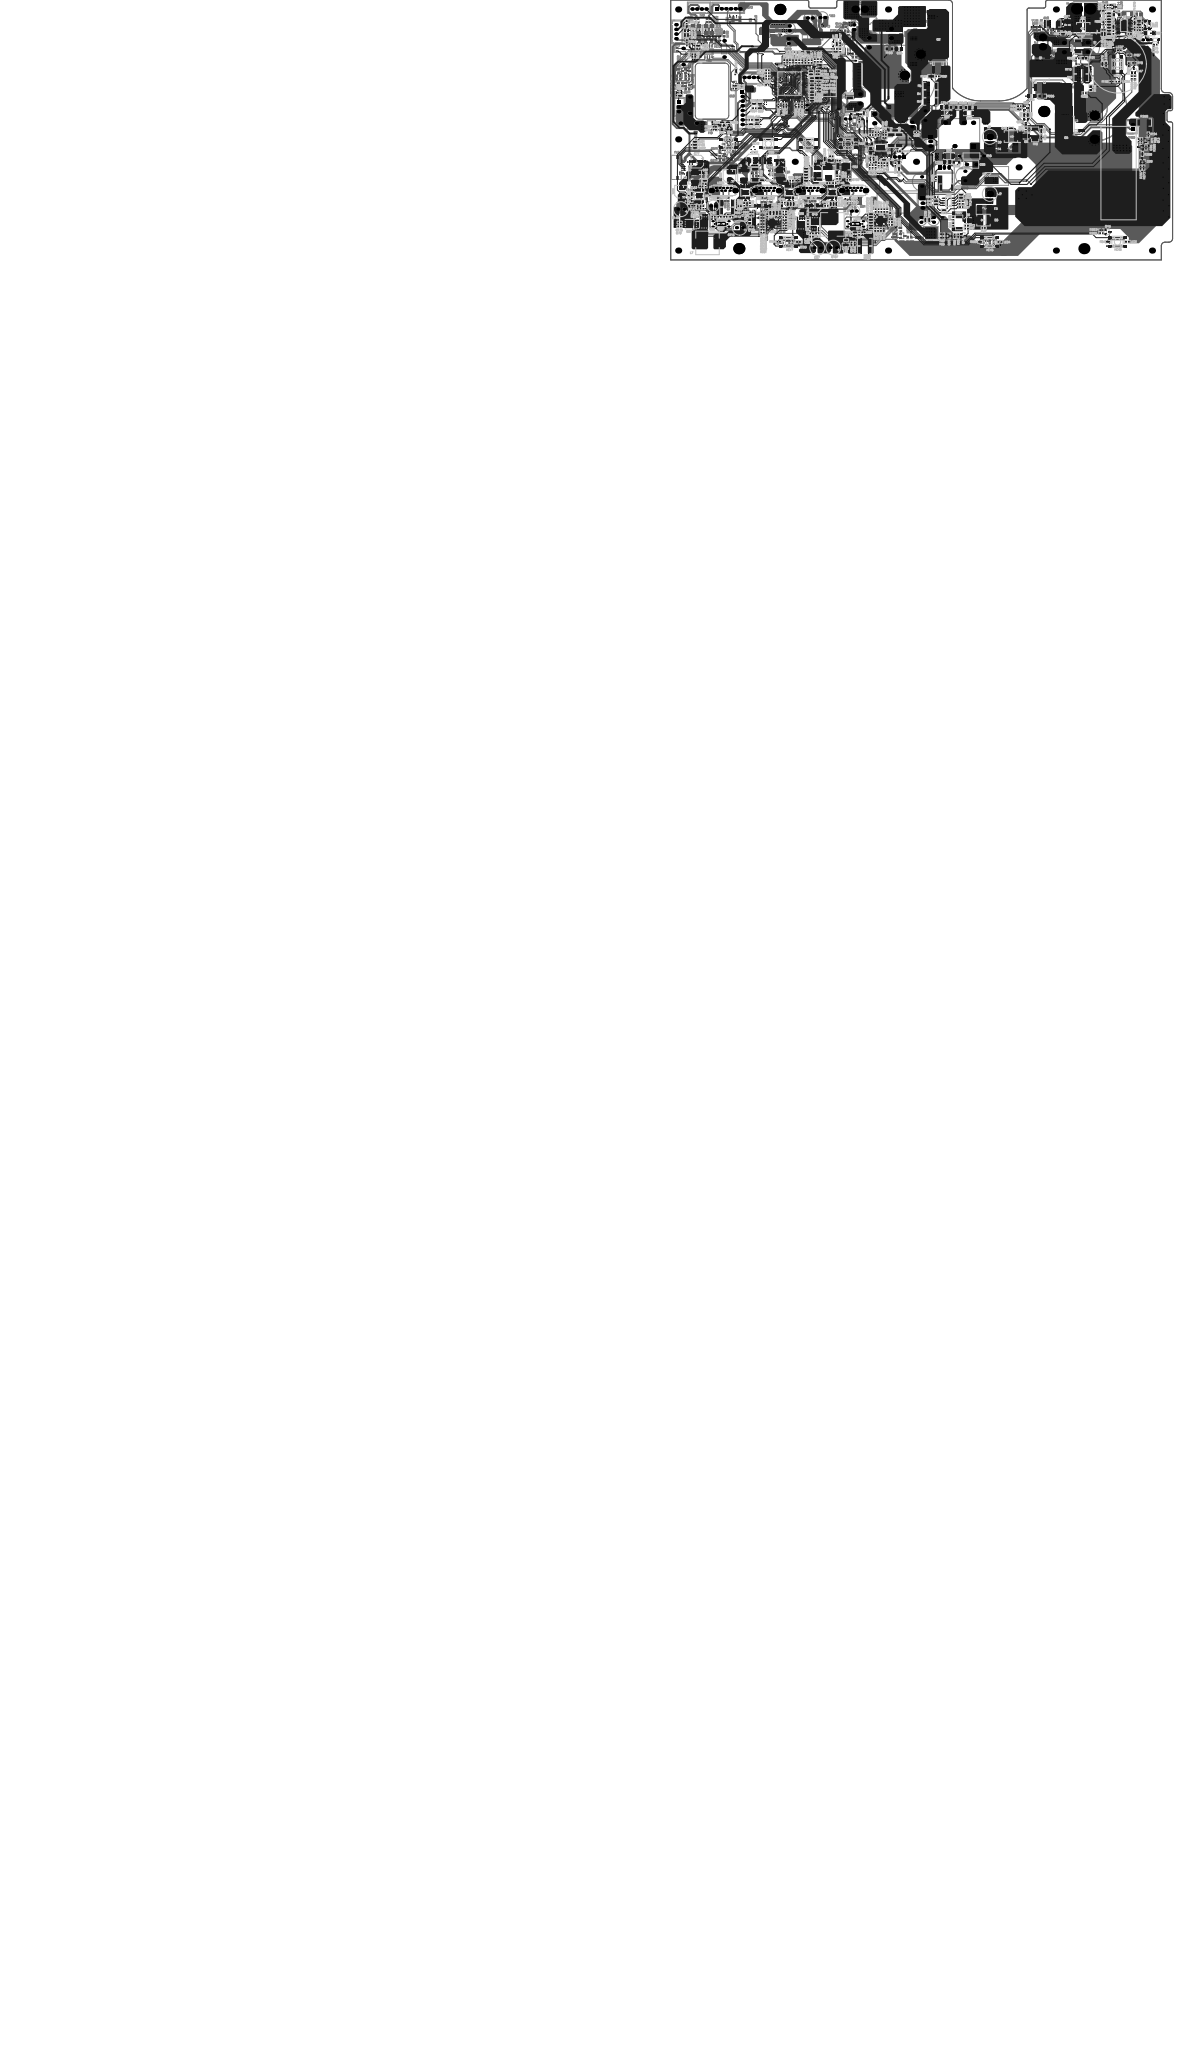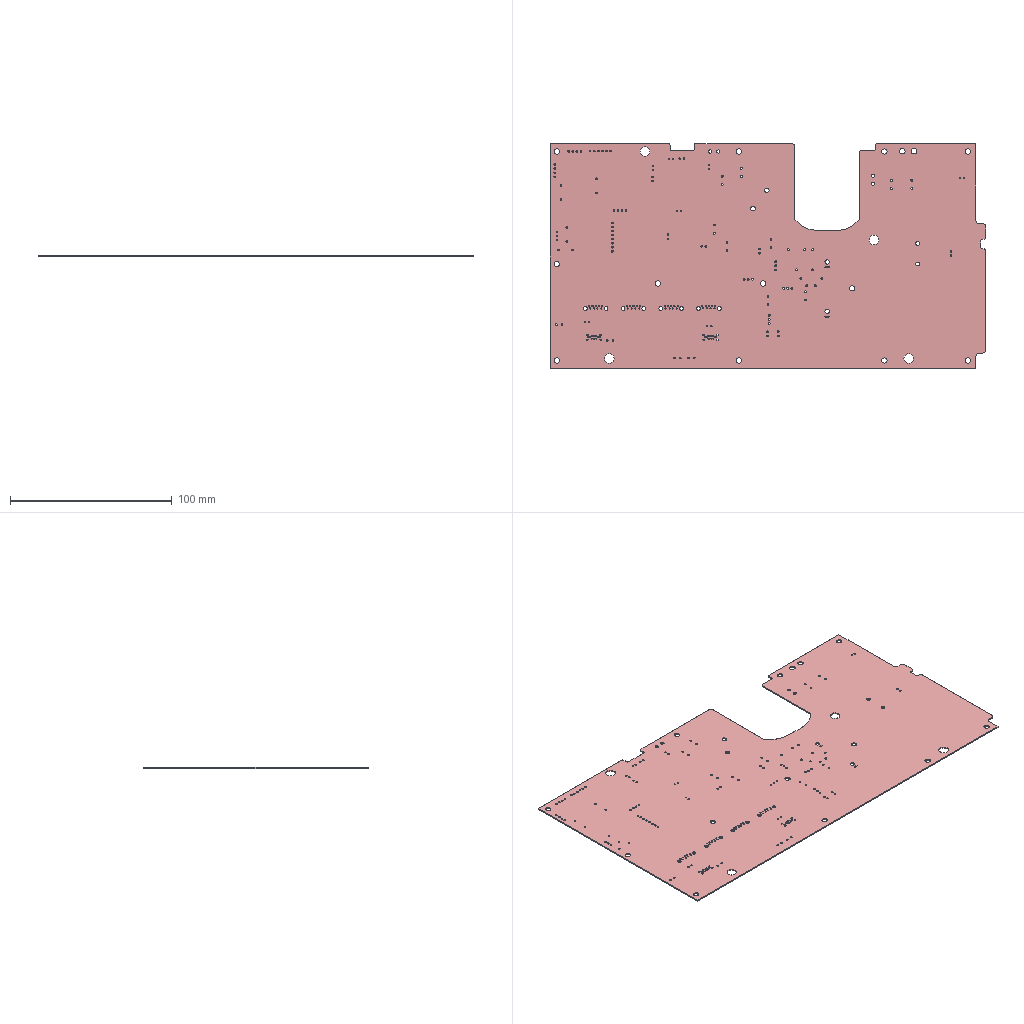Circuit board layout | Altium Designer | box 269.1 x 139 x 0.8 mm
Layer stack:
# Altium Designer layer stack of  (unit mm; dielectric type: 0 none, 1 core, 2 prepreg, 3 surface material)
index,name,kind,layer,copper_thickness_mm,dielectric_type,dielectric_thickness_mm,dielectric_material,dielectric_constant
0,Top Paste,other,,,,,,
1,Top Overlay,other,,,,,,
2,Top Solder,dielectric,,,3,0.0102,Solder Resist,3.5
3,TOP,copper,TOP,0.0305,,,,
4,Dielectric1,dielectric,,,1,0.2032,FR-4,4.5
5,GND02,copper,GND02,0.0305,,,,
6,Dielectric2,dielectric,,,1,0.2032,FR-4,4.5
7,PWR03,copper,PWR03,0.0305,,,,
8,Dielectric3,dielectric,,,1,0.2032,FR-4,4.5
9,BOTTOM,copper,BOTTOM,0.0305,,,,
10,Bottom Solder,dielectric,,,3,0.0102,Solder Resist,3.5
11,Bottom Overlay,other,,,,,,
12,Bottom Paste,other,,,,,,
# drill layer pairs: low layer,high layer
drill_pair,TOP,BOTTOM
Part placement, first 577 of 695 lines:
Designator,Comment,Layer,Footprint,Center-X(mm),Center-Y(mm),Rotation
C189,100uF,TopLayer,CAP-TH_BD6.3-P2.50-D1.0-FD,98.18,26.138,0
C188,100uF,TopLayer,CAP-TH_BD6.3-P2.50-D1.0-FD,22.724,28.837,180
R189,,TopLayer,R0603,61.155,22.826,360
Q2,CRSS042N10N,TopLayer,TO-263-3_L10.2-W10.7-P5.08-LS16.2-TL,143.332,106.96,90
R368,15,TopLayer,r2512,253.805,73.517,180
C160,100uF,TopLayer,CAP-SMD_BD6.3-L6.6-W6.6-FD,77.614,47.26,270
C130,56pF,TopLayer,C0603,114.3,53.594,180
CON1,HX25003-2A,BottomLayer,CONN-TH_2P-P2.50_HX25003-2A,247.575,71.181,90
R29,,TopLayer,R0603,152.187,12.886,270
U7,L7805CV-DG,BottomLayer,TO-220-3_L10.0-W4.5-P2.54-L,135.239,30.336,270
R353,2K,BottomLayer,R0603,203.217,123.072,360
R352,10K,BottomLayer,R0603,203.217,121.421,360
R351,20K,BottomLayer,R0603,128.711,15.858,270
R350,20K,BottomLayer,R0603,120.261,12.226,360
R349,,BottomLayer,R0603,120.277,13.859,180
R348,,BottomLayer,R0603,127.982,12.049,360
R338,,BottomLayer,R0603,123.199,16.341,270
R337,2K,BottomLayer,R0603,171.992,9.897,180
R336,10K,BottomLayer,R0603,172,8.34,360
R335,2K,BottomLayer,R0603,64.448,8.297,180
R334,10K,BottomLayer,R0603,64.457,9.864,360
R333,2K,TopLayer,R0603,247.227,97.629,90
R332,10K,TopLayer,R0603,248.86,97.621,270
R325,2K,TopLayer,R0603,230.852,14.342,360
R323,10K,TopLayer,R0603,230.869,15.96,180
R317,,TopLayer,R0603,75.574,106.113,90
R314,2K,BottomLayer,R0603,235.881,135.374,90
R308,10K,BottomLayer,R0603,237.862,135.424,90
R302,2K,TopLayer,R0603,232.571,135.501,90
R297,10K,TopLayer,R0603,234.204,135.517,270
R291,2K,BottomLayer,R0603,99.704,55.253,270
R289,2K,TopLayer,R0603,254.778,60.13,270
R288,10K,TopLayer,R0603,252.866,56.684,90
R287,2K,TopLayer,R0603,251.875,49.344,90
R286,,BottomLayer,R0603,75.751,97.374,180
R285,,BottomLayer,R0603,72.221,104.131,180
R284,,BottomLayer,R0603,75.353,101.66,360
R282,,TopLayer,R0603,78.859,100.981,360
R280,,TopLayer,R0603,75.192,99.247,180
R279,,BottomLayer,R0603,84.04,34.485,90
R278,,BottomLayer,R0603,60.621,33.316,90
R277,,BottomLayer,R0603,37.659,33.037,90
R273,,TopLayer,R0603,11.261,32.148,90
R272,10K,TopLayer,R0603,253.534,49.361,270
Q53,SS8050_C2898656,BottomLayer,SOT-23-3_L2.9-W1.3-P1.90-LS2.4-BR,198.847,123.766,180
Q52,SS8550_C2762207,BottomLayer,SOT-23-3_L2.9-W1.3-P1.90-LS2.4-BR,206.925,122.343,180
Q51,SS8050_C2898656,BottomLayer,SOT-23-3_L2.9-W1.3-P1.90-LS2.4-BR,124.197,12.946,180
Q50,HSU4103,BottomLayer,TO-252-2_L6.6-W6.1-P4.57-LS9.9-BR,135.988,14.309,90
Q49,SS8050_C2898656,BottomLayer,SOT-23-3_L2.9-W1.3-P1.90-LS2.4-BR,168.411,8.949,360
Q48,SS8050_C2898656,BottomLayer,SOT-23-3_L2.9-W1.3-P1.90-LS2.4-BR,60.842,8.924,360
Q47,SS8050_C2898656,TopLayer,SOT-23-3_L2.9-W1.3-P1.90-LS2.4-BR,248.175,101.489,270
Q46,SS8050_C2898656,TopLayer,SOT-23-3_L2.9-W1.3-P1.90-LS2.4-BR,234.28,15.02,180
Q45,SS8550_C2762207,BottomLayer,SOT-23-3_L2.9-W1.3-P1.90-LS2.4-BR,232.902,135.289,360
Q44,SS8050_C2898656,BottomLayer,SOT-23-3_L2.9-W1.3-P1.90-LS2.4-BR,95.648,56.346,90
Q39,SS8050_C2898656,TopLayer,SOT-23-3_L2.9-W1.3-P1.90-LS2.4-BR,252.849,53.026,270
Q36,SS8550_C2762207,TopLayer,SOT-23-3_L2.9-W1.3-P1.90-LS2.4-BR,251.85,60.24,360
Q31,SS8550_C2762207,TopLayer,SOT-23-3_L2.9-W1.3-P1.90-LS2.4-BR,27.44,70.697,90
Q21,SS8050_C2898656,TopLayer,SOT-23-3_L2.9-W1.3-P1.90-LS2.4-BR,190.389,81.263,180
Q19,SS8050_C2898656,TopLayer,SOT-23-3_L2.9-W1.3-P1.90-LS2.4-BR,149.114,12.81,180
LED7,LED-0603_R,TopLayer,LED0603_RED,240.479,112.081,360
LED6,LED-0603_R,TopLayer,LED0603_RED,239.734,95.437,180
LED5,LED-0603_R,TopLayer,LED0603_RED,233.384,104.639,90
D13,RS1DG,TopLayer,SMA_L4.4-W2.8-LS5.4-RD,159.647,78.546,180
C76,220uF,BottomLayer,CAP-TH_BD6.3-P2.50-D1.0-FD,140.877,21.454,270
C75,680uF,BottomLayer,CAP-TH_BD10.0-P5.00-D1.0-FD,134.535,41.919,90
C74,100nF,BottomLayer,C0603,75.684,95.742,360
C73,100nF,BottomLayer,C0603,72.001,102.523,360
C52,100nF,BottomLayer,C0603,75.531,103.514,360
C35,100nF,TopLayer,C0603,75.142,100.923,180
C34,100nF,TopLayer,C0603,77.232,106.688,270
C17,220pF,BottomLayer,C0603,84.04,38.015,90
C8,220pF,BottomLayer,C0603,60.621,36.458,90
C7,220pF,BottomLayer,C0603,37.66,36.28,90
C3,220pF,TopLayer,C0603,11.261,35.315,90
J1,TJC1-2A,TopLayer,CONN-TH_XT30UPB-F-W,199.314,116.52,90
C24,100nF,TopLayer,C0603,248.666,123.698,90
C27,100nF,TopLayer,C0603,250.952,125.857,180
C1,100nF,TopLayer,C0603,234.95,130.302,180
R12,,TopLayer,R0603,234.95,131.927,360
R49,,TopLayer,R0603,250.943,122.936,180
C25,4.7nF,TopLayer,C1206,122.301,112.903,180
D41,MM3Z3V3_C123917,TopLayer,SOD-323_L1.8-W1.3-LS2.5-RD,87.249,115.57,90
C159,100nF,TopLayer,C0603,89,115.443,90
R295,1K,TopLayer,R0603,88.392,112.903,360
R107,,TopLayer,R0603,90.805,115.443,270
R294,,TopLayer,R0603,90.805,112.141,270
R75,,TopLayer,R0603,88.392,111.379,180
R206,,TopLayer,R1206,199.119,87.63,360
R198,,TopLayer,R1206,117.221,112.903,180
R186,2K,BottomLayer,R0603,31.242,70.002,180
R148,,TopLayer,R0603,122.292,58.191,360
R137,100,BottomLayer,R0603,95.25,31.166,90
R125,,TopLayer,R0805,225.171,91.855,90
R120,100,BottomLayer,R0603,50.698,31.953,90
R118,2K,TopLayer,R0603,236.271,95.453,180
R116,,TopLayer,R0603,100.965,13.97,270
R115,,TopLayer,R0603,98.806,12.954,360
R114,,TopLayer,R0603,26.171,23.114,180
R113,,TopLayer,R0603,32.503,23.114,360
R110,0.01,TopLayer,R2512,220.109,101.6,180
R104,10K,BottomLayer,R0603,98.146,55.27,270
R102,100,BottomLayer,R0603,52.197,31.956,90
R101,,TopLayer,R0805,139.615,98.222,180
LED4,LED-0603_R,TopLayer,LED0603_RED,176.479,9.601,180
C42,680pF,TopLayer,C0603,108.204,50.038,90
C37,3.9nF,TopLayer,C0603,234.925,125.806,180
R54,,TopLayer,R1206,107.188,58.359,90
C36,4.7nF,TopLayer,C1206,193.404,87.63,360
Q20,SS8550_C2762207,TopLayer,SOT-23-3_L2.9-W1.3-P1.90-LS2.4-BR,190.435,73.879,90
U19,TL431_C2688223,TopLayer,SOT-23-3_L2.9-W1.6-P1.90-LS2.8-BR-CW,78.512,103.47,360
U13,GD32F103VCT6,TopLayer,LQFP-100_L14.0-W14.0-P0.50-LS16.0-BL,63.653,94.326,90
U29,UC2845BD1013TR,TopLayer,SOP-8_L4.9-W3.9-P1.27-LS6.0-BL,148.854,31.08,90
U22,SW3521,TopLayer,ESOP-8_L4.9-W3.9-P1.27-LS6.0-BL-EP,86.513,36.287,180
U6,SW3521,TopLayer,ESOP-8_L4.9-W3.9-P1.27-LS6.0-BL-EP,63.526,36.287,180
U5,SW3521,TopLayer,ESOP-8_L4.9-W3.9-P1.27-LS6.0-BL-EP,15.193,34.255,180
U4,SW3521,TopLayer,ESOP-8_L4.9-W3.9-P1.27-LS6.0-BL-EP,40.031,36.16,180
U2C,Value,TopLayer,QFN-28_L4.0-W4.0-P0.40-BL-EP,54.382,19.777,180
U1C,Value,TopLayer,QFN-28_L4.0-W4.0-P0.40-BL-EP,112.421,21.047,270
U1,LM5116MHX,TopLayer,HTSSOP-20_L6.5-W4.4-P0.65-LS6.4-BL-EP,242.951,125.476,270
R16,15K,TopLayer,RES-TH_BD3.3-L9.0-P13.00-D0.6,161.212,55.591,360
R316,0.15,TopLayer,R2512,147.835,38.7,0
R266,0.01,TopLayer,R2512,104.021,9.617,360
R262,0.01,TopLayer,R2512,30.208,30.353,180
R227,,TopLayer,RES-SMD_L6.4-W3.2-R2512,154.618,20.066,180
R169,0.01,TopLayer,R2512,104.021,5.299,360
R83,,TopLayer,R2512,92.482,50.13,180
R41,,TopLayer,R2512,139.323,84.709,360
R28,,TopLayer,R2512,45.289,45.583,90
R26,,TopLayer,R2512,205.262,126.496,360
R19,,TopLayer,RES-SMD_L6.4-W3.2-R2512,195.334,67.157,360
R18,0.01,TopLayer,R2512,220.109,97.409,180
R5,,TopLayer,R2512,139.323,93.091,360
R4,,TopLayer,R2512,139.323,88.9,360
Q43,HSBA6040,TopLayer,POWERPAK-SO-8_L6.2-W5.2-P1.27-BR-EP,77.242,19.586,270
Q38,HSBA6040,TopLayer,POWERPAK-SO-8_L6.2-W5.2-P1.27-BR-EP,17.933,20.081,90
Q37,HSBA6040,TopLayer,POWERPAK-SO-8_L6.2-W5.2-P1.27-BR-EP,10.757,19.142,360
Q28,HSBA6040,TopLayer,POWERPAK-SO-8_L6.2-W5.2-P1.27-BR-EP,69.876,19.573,90
Q25,SS8050_C2898656,TopLayer,SOT-23-3_L2.9-W1.3-P1.90-LS2.4-BR,31.41,71.069,270
Q29,AP050N03Q,TopLayer,PDFN-8_L3.1-W3.1-P0.65-LS3.4-BL,212.66,123.835,270
Q27,AP050N03Q,TopLayer,PDFN-8_L3.1-W3.1-P0.65-LS3.4-BL,212.66,127.518,270
Q9,AP050N03Q,TopLayer,PDFN-8_L3.1-W3.1-P0.65-LS3.4-BL,159.569,21.042,270
Q6,AP050N03Q,TopLayer,PDFN-8_L3.1-W3.1-P0.65-LS3.4-BL,190.495,66.263,90
Q5,CRSS042N10N,TopLayer,TO-263-3_L10.2-W10.7-P5.08-LS16.2-TL,215.292,71.882,180
Q1,CRSS042N10N,TopLayer,TO-263-3_L10.2-W10.7-P5.08-LS16.2-TL,197.866,97.255,90
LED3,LED-0603_R,TopLayer,LED0603_RED,68.478,9.627,180
LED2,LED-0603_R,TopLayer,LED0603_RED,245.567,104.496,90
LED1,LED-0603_R,TopLayer,LED0603_RED,244.805,9.754,180
L13,BLM21PG300SN1D,TopLayer,L0805,93.853,8.001,360
L12,BLM21PG300SN1D,TopLayer,L0805,42.291,20.651,90
L7,10uH,TopLayer,IND-SMD_L13.8-W12.6_YSPI13XX,19.711,9.109,0
L6,10uH,TopLayer,IND-SMD_L13.8-W12.6_YSPI13XX,86.665,18.998,270
L10,22uH,TopLayer,IND-SMD_L7.1-W6.8,84.735,46.828,90
L9,22uH,TopLayer,IND-SMD_L7.1-W6.8,58.573,45.812,90
L5,22uH,TopLayer,IND-SMD_L7.1-W6.8,39.269,45.437,90
L3,22uH,TopLayer,IND-SMD_L7.1-W6.8,13.081,44.323,90
J13,TJC1-2A,TopLayer,CONN-TH_XT30UPB-F-W,101.336,134.086,180
J4,TJC1-2A,TopLayer,CONN-TH_XT60UPB-F-W,221.126,134.239,360
F2,FUSE/20A,TopLayer,FUSE-SMD_L6.1-W2.5,228.346,121.92,90
F6,5A/125V,TopLayer,FUSE-SMD_L6.1-W2.5,171.095,45.729,90
F4,FUSE/5A,TopLayer,FUSE-SMD_L6.1-W2.5,181.807,59.528,180
F3,FUSE/5A,TopLayer,FUSE-SMD_L6.1-W2.5,168.091,27.651,360
D62,RS1DG,TopLayer,SMA_L4.4-W2.8-LS5.4-RD,148.006,78.705,0
D48,MMSZ5242B_R1_00001,TopLayer,SOD-123_L2.7-W1.6-LS3.7-RD-1,122.403,50.538,270
D20,ES3DB,TopLayer,SMB_L4.6-W3.6-LS5.3-RD,149.071,55.591,180
D57,MM3Z3V3_C123917,TopLayer,SOD-323_L1.8-W1.3-LS2.5-RD,4.471,89.5,180
D9,SS34,TopLayer,SMC_L7.1-W6.2-LS8.1-R-RD,182.392,66.005,360
D8,SS34,TopLayer,SMC_L7.1-W6.2-LS8.1-R-RD,167.672,21.301,180
D7,SS34,TopLayer,SMC_L7.1-W6.2-LS8.1-R-RD,221.158,123.876,180
C140,220uF,TopLayer,CAP-TH_BD8.0-P3.50-D0.6-FD,5.515,27.143,180
C115,220uF,TopLayer,CAP-TH_BD8.0-P3.50-D0.6-FD,36.983,17.265,180
C107,220uF,TopLayer,CAP-TH_BD8.0-P3.50-D0.6-FD,87.176,6.569,180
C97,220uF,TopLayer,CAP-TH_BD8.0-P3.50-D0.6-FD,78.54,6.442,360
C174,10nF,BottomLayer,C0603,64.288,30,90
C122,100uF,TopLayer,CAP-SMD_BD6.3-L6.6-W6.6-FD,43.812,53.213,360
C95,100uF,TopLayer,CAP-SMD_BD6.3-L6.6-W6.6-FD,54.737,53.213,180
C77,100uF,TopLayer,CAP-SMD_BD6.3-L6.6-W6.6-FD,14.224,52.578,180
C399,100nF,TopLayer,C0603,75.56,14.241,180
C194,15nF,TopLayer,C0603,237.363,124.714,90
C176,100nF,TopLayer,C0603,4.787,20.031,360
C168,100nF,TopLayer,C0603,12.954,61.595,360
C162,100nF,TopLayer,C0603,83.4,28.921,180
C161,100nF,TopLayer,C0603,60.413,30.699,180
C151,100nF,TopLayer,C0603,84.481,41.113,180
C150,100nF,TopLayer,C0603,90.069,53.178,180
C148,100nF,TopLayer,C0603,87.656,41.113,180
C147,100nF,TopLayer,C0603,12.091,29.048,180
C143,100nF,TopLayer,C0603,16.347,39.335,180
C142,100nF,BottomLayer,C0603,56.449,43.662,360
C118,100nF,TopLayer,C0603,14.696,114.646,180
C90,100nF,TopLayer,C0603,43.219,25.502,180
C84,100nF,TopLayer,C0603,96.901,8.636,270
C83,100nF,TopLayer,C0603,98.679,8.636,270
C80,100nF,TopLayer,C0603,98.806,14.732,180
C68,100nF,TopLayer,C0603,64.796,42.383,180
C67,100nF,TopLayer,C0603,155.728,28.286,180
C62,1nF,TopLayer,C0603,18.274,42.383,360
C60,100nF,TopLayer,C0603,36.983,28.794,180
C57,100nF,BottomLayer,C0603,37.795,48.768,360
C56,100nF,TopLayer,C0603,198.654,68.99,270
C53,100nF,TopLayer,C0603,151.41,19.015,90
C40,100nF,TopLayer,C0603,142.266,31.461,0
C30,220uF,BottomLayer,CAP-TH_BD6.3-P2.50-D1.0-FD,134.137,21.428,270
C29,1nF,TopLayer,C0603,72.543,48.86,180
C18,56pF,TopLayer,C0603,237.363,121.666,90
C14,2.2nF,TopLayer,C0603,116.129,51.13,90
J3,TJC1-2A,TopLayer,DC5521,171.049,64.199,0
J2,TJC1-2A,TopLayer,DC5521,171.049,33.7,0
KEY8,4-1437565-2,TopLayer,SW-SMD_4P-L6.0-W6.0-P4.50-LS8.6,239.5,9.67,0
KEY5,4-1437565-2,TopLayer,SW-SMD_4P-L6.0-W6.0-P4.50-LS8.6,171,9.669,0
KEY6,4-1437565-2,TopLayer,SW-SMD_4P-L6.0-W6.0-P4.50-LS8.6,239.548,104.75,90
KEY7,4-1437565-2,TopLayer,SW-SMD_4P-L6.0-W6.0-P4.50-LS8.6,62.999,9.669,0
KEY4,4-1437565-2,TopLayer,SW-SMD_4P-L6.0-W6.0-P4.50-LS8.6,95.099,62.169,0
KEY3,4-1437565-2,TopLayer,SW-SMD_4P-L6.0-W6.0-P4.50-LS8.6,73.763,62.169,0
KEY2,4-1437565-2,TopLayer,SW-SMD_4P-L6.0-W6.0-P4.50-LS8.6,52.3,62.169,0
R324,1K,TopLayer,R0603,60.478,82.515,90
R258,1K,TopLayer,R0603,155.601,33.239,180
R240,22,TopLayer,R0603,142.266,33.62,180
R200,1K,TopLayer,R0603,61.13,16.984,360
R199,1K,TopLayer,R0603,61.13,18.381,360
R195,2K,TopLayer,R0603,165.76,9.652,360
R194,2K,TopLayer,R0603,57.937,9.754,360
R187,2K,TopLayer,R0603,245.821,109.55,360
R135,,TopLayer,R0603,65.812,29.945,90
R134,49.9K,TopLayer,R0603,156.617,30.707,90
R133,,TopLayer,R0603,42.444,29.818,90
R132,,TopLayer,R0603,17.479,28.18,90
R131,,TopLayer,R0603,78.512,14.316,180
R130,,TopLayer,R0603,117.991,18.761,360
R129,,TopLayer,R0603,117.991,20.285,360
R128,1K,TopLayer,R0603,117.991,21.809,360
R127,1K,TopLayer,R0603,117.602,24.511,90
R122,,TopLayer,R0603,61.157,24.401,360
R111,100,TopLayer,R0603,62.764,29.945,90
R103,1K,TopLayer,R0603,18.745,39.998,90
R70,1K,TopLayer,R0603,198.654,65.488,90
R69,1K,TopLayer,R0603,151.41,22.317,270
R66,,TopLayer,R0603,190.444,69.865,270
R65,10K,TopLayer,R0603,145.515,11.887,180
R61,,TopLayer,R0603,158.722,16.779,180
R47,1K,TopLayer,R0603,62.002,82.523,90
R44,,TopLayer,R0603,186.795,82.219,180
R43,,BottomLayer,R0603,113.021,62.941,180
R42,,TopLayer,R0603,23.648,69.688,180
R40,2K,TopLayer,R0603,186.813,80.544,360
R23,2K,TopLayer,R0603,154.102,12.944,90
R21,,TopLayer,R0603,246.126,120.904,180
R20,49.9K,TopLayer,R0603,120.447,51.044,90
R8,27K,TopLayer,R0603,114.427,51.181,270
R2,NC,TopLayer,R0603,111.379,67.564,90
R1,,TopLayer,R1206,239.014,131.191,180
R341,,TopLayer,R0603,67.97,42.428,180
R339,,TopLayer,R0603,89.179,44.104,270
R322,,TopLayer,R0603,12.954,59.944,360
R321,,TopLayer,R0603,12.954,63.246,180
R309,,TopLayer,R0603,109.881,26.389,270
R307,,TopLayer,R0603,61.156,25.823,180
R306,,TopLayer,R0603,234.95,122.682,180
R298,,TopLayer,R0603,4.97,87.849,360
R293,,TopLayer,R0603,75.718,91.786,360
R292,,TopLayer,R0603,88.799,29.937,90
R283,,TopLayer,R0603,51.85,96.866,360
R274,NC,TopLayer,R0603,248.666,126.746,270
R265,,TopLayer,R0603,142.139,43.78,90
R261,,TopLayer,R0603,143.078,98.222,180
R259,,TopLayer,R0603,221.86,89.281,360
R252,,TopLayer,R0603,75.709,85.182,360
R251,,TopLayer,R0603,68.606,82.523,270
R250,,TopLayer,R0603,67.082,82.523,270
R249,,TopLayer,R0603,51.85,101.438,360
R247,100,TopLayer,R0603,85.751,29.945,90
R246,,TopLayer,R0603,51.85,99.914,360
R245,100,TopLayer,R0603,87.275,29.945,90
R243,100,TopLayer,R0603,14.431,28.18,90
R242,100,TopLayer,R0603,15.955,28.18,90
R241,,TopLayer,R0603,90.703,44.028,270
R238,100,TopLayer,R0603,64.288,29.945,90
R229,,TopLayer,R0603,14.767,112.868,180
R228,,TopLayer,R0603,70.384,82.523,270
R224,,TopLayer,R0603,62.383,106.264,270
R222,,TopLayer,R0603,57.684,82.506,270
R221,,TopLayer,R0603,75.709,89.754,360
R219,,TopLayer,R0603,75.709,88.23,360
R218,NC,TopLayer,R0603,49.165,17.637,180
R217,,TopLayer,R0603,51.715,93.691,180
R216,,TopLayer,R0603,49.184,19.142,360
R215,,TopLayer,R0603,49.184,20.92,360
R214,,TopLayer,R0603,49.184,22.444,360
R213,,TopLayer,R0603,49.168,24.003,360
R211,,TopLayer,R0603,51.715,23.824,270
R202,,TopLayer,R0603,49.209,16.146,180
R201,,TopLayer,R0603,49.218,14.622,180
R196,,TopLayer,R0603,111.405,26.372,270
R185,NC,TopLayer,R0603,61.148,21.328,360
R183,,TopLayer,R0603,23.648,71.212,180
R182,NC,TopLayer,R0603,61.148,19.804,360
R181,NC,TopLayer,R0603,114.223,16.097,270
R179,,TopLayer,R0603,112.675,16.094,90
R178,,TopLayer,R0603,111.151,16.102,90
R175,,TopLayer,R0603,109.627,16.085,90
R174,,TopLayer,R0603,73.559,21.555,90
R173,,TopLayer,R0603,107.35,16.856,360
R172,,TopLayer,R0603,192.095,69.815,270
R170,,TopLayer,R0603,107.35,18.38,360
R162,NC,TopLayer,R0603,115.977,26.372,90
R161,NC,TopLayer,R0603,114.453,26.372,90
R156,,TopLayer,R0603,13.107,109.32,90
R154,,TopLayer,R0603,11.583,109.32,90
R151,,TopLayer,R0603,112.929,26.372,90
R150,,TopLayer,R0603,75.709,86.706,360
R94,,TopLayer,R0603,51.85,98.339,360
R89,100,TopLayer,R0603,39.396,29.818,90
R87,,TopLayer,R0603,72.491,44.053,360
R81,100,TopLayer,R0603,40.92,29.818,90
R72,,TopLayer,R0603,158.722,18.253,360
R62,1K,TopLayer,R0603,72.517,47.152,180
R58,1K,TopLayer,R0603,72.543,45.558,360
R55,,TopLayer,R0603,251.07,127.889,180
R48,,TopLayer,R0603,259.7,115.215,180
R32,2K,TopLayer,R0603,145.5,13.777,360
R15,,TopLayer,R0603,109.855,67.564,270
R14,,TopLayer,R0603,113.03,51.181,270
R13,AC2512FK-073KL,TopLayer,R2512,118.237,64.049,270
R10,,TopLayer,R0603,234.95,128.749,360
R3,,TopLayer,R0603,60.859,106.264,270
C199,10uF,TopLayer,C0603,95.377,42.926,180
C170,10uF,TopLayer,C0603,72.543,42.383,180
C164,20pF,TopLayer,C0603,75.718,93.437,180
C146,100pF,TopLayer,C0603,107.279,19.904,180
C141,10uF,TopLayer,C0603,22.962,23.165,360
C135,390pF,TopLayer,C0603,107.279,22.952,180
C134,100pF,TopLayer,C0603,53.366,25.175,90
C129,10uF,TopLayer,C0603,43.18,17.399,180
C119,2.2nF,TopLayer,C0603,73.559,18.507,90
C113,10uF,TopLayer,C0603,94.006,10.633,180
C111,390pF,TopLayer,C0603,56.922,25.175,90
C109,100pF,TopLayer,C0603,55.144,25.175,90
C108,100pF,TopLayer,C0603,107.279,21.428,180
C98,10nF,TopLayer,CAP-TH_L8.0-W4.0-P5.00-D1.2,161.096,51.071,0
C88,10uF,TopLayer,C0603,103.339,14.824,360
C81,1nF,TopLayer,C0603,154.839,30.699,90
C79,2.2uF,TopLayer,C0603,4.699,17.907,360
C55,2.2uF,TopLayer,C0603,75.56,12.463,180
C49,10uF,TopLayer,C0603,48.921,42.637,180
C48,10uF,TopLayer,C0603,182.463,70.323,180
C47,10uF,TopLayer,C0603,167.793,17.11,360
C33,1uF,TopLayer,C0603,107.569,66.802,360
C21,100nF,TopLayer,C0603,73.889,106.121,270
C10,1uF,TopLayer,C0603,248.666,129.667,270
KEY1,4-1437565-2,TopLayer,SW-SMD_4P-L6.0-W6.0-P4.50-LS8.6,30.964,62.169,0
R25,,TopLayer,R0603,115.316,67.564,270
R27,,TopLayer,R0603,250.943,124.398,180
C127,100nF,TopLayer,C0603,75.702,95.723,180
C126,100nF,TopLayer,C0603,79.258,93.437,180
R176,1K,TopLayer,R0603,34.325,91.659,180
R163,100K,TopLayer,NTC,79.35,97.424,360
R57,100K,TopLayer,NTC,72.806,81.484,90
R257,,TopLayer,R0603,75.718,97.247,180
R256,,TopLayer,R0603,79.384,91.659,180
R203,,TopLayer,R0603,58.573,25.229,270
R160,,TopLayer,R0603,107.329,24.476,360
R157,,TopLayer,R0603,35.078,101.065,270
R146,,TopLayer,R0603,34.307,93.183,180
R46,,TopLayer,R0603,79.274,95.596,360
R33,,TopLayer,R0603,79.4,90.053,360
C96,100nF,TopLayer,C0603,131.693,68.25,360
C45,100nF,TopLayer,C0603,142.25,29.683,180
R39,,TopLayer,R0603,191.439,77.556,90
R35,2K,TopLayer,R0603,189.484,77.562,90
R9,120K,TopLayer,R0603,101.092,74.549,90
R117,8.25K,TopLayer,R0603,146.481,26.594,180
C89,1nF,TopLayer,C0603,155.654,34.976,0
R331,,TopLayer,R1206,106.426,62.103,360
Q14,SS8550_C2762207,TopLayer,SOT-23-3_L2.9-W1.3-P1.90-LS2.4-BR,157.032,13.047,180
USB1,TYPE-C2022512,TopLayer,NEW_TYPEC,26.98,19.269,180
USB6,TYPE-C2022512,TopLayer,NEW_TYPEC,99.121,19.269,180
R296,2K,TopLayer,R0603,231.927,126.619,90
USB2,916-252A205IY30200,TopLayer,USB-A-TH_916-252A205IY30200,51.41,37.772,360
USB3,916-252A205IY30200,TopLayer,USB-A-TH_916-252A205IY30200,74.715,37.772,360
USB4,916-252A205IY30200,TopLayer,USB-A-TH_916-252A205IY30200,98.007,37.823,360
USB5,916-252A205IY30200,TopLayer,USB-A-TH_916-252A205IY30200,28.098,37.797,360
R267,0.01,TopLayer,R2512,30.208,26.162,180
C138,100nF,TopLayer,C0603,43.219,23.749,180
C91,100nF,TopLayer,C0603,29.272,23.114,360
C16,100nF,TopLayer,C0603,114.554,65.278,180
C15,100nF,TopLayer,C0603,108.712,54.102,270
R223,,TopLayer,R0603,107.061,54.102,90
C13,15nF,TopLayer,C0603,111.506,51.181,270
R11,,TopLayer,R0603,106.68,50.038,90
C12,1nF,TopLayer,C0603,109.855,50.038,90
R22,,TopLayer,R0603,113.919,67.564,270
U3,LM5116MHX,TopLayer,HTSSOP-20_L6.5-W4.4-P0.65-LS6.4-BL-EP,112.522,60.071,360
R64,2K,TopLayer,R0603,234.442,9.728,360
D52,1SMA4742A_C382772,TopLayer,SMA_L4.4-W2.6-LS5.0-RD,256.794,121.285,0
D23,FR107_C2760867,TopLayer,SOD-123FL_L2.7-W1.8-LS3.8-RD,256.54,125.73,90
C20,2.2nF,TopLayer,C0603,234.95,120.777,180
R248,36K,TopLayer,R0603,232.664,120.904,270
R136,,TopLayer,R0603,231.267,120.904,270
R56,,TopLayer,R0603,210.312,120.98,360
R34,,TopLayer,R0603,232.029,123.063,360
C41,10uF,TopLayer,C0603,220.853,127.889,360
R52,,TopLayer,R0603,234.95,127.381,360
R51,2K,BottomLayer,R0603,105.308,53.848,90
R84,100,BottomLayer,R0603,73.965,32.334,90
R121,,TopLayer,R0805,221.776,107.95,360
D21,FR107_C2760867,TopLayer,SOD-123FL_L2.7-W1.8-LS3.8-RD,254.381,125.73,270
R253,,TopLayer,R0603,218.059,107.95,360
C59,100nF,TopLayer,C0603,47.814,83.566,180
C69,100nF,TopLayer,C0603,47.817,81.153,180
C71,100nF,TopLayer,C0603,46.166,74.93,180
C72,100nF,TopLayer,C0603,46.166,72.517,180
F5,10A/100V,TopLayer,FUSE-SMD_L6.1-W2.5,204.629,109.322,360
R207,,TopLayer,R0603,44.641,83.569,180
R254,,TopLayer,R0603,44.764,81.128,180
R255,,TopLayer,R0603,42.917,74.93,180
R264,,TopLayer,R0603,43.044,72.517,180
R269,,TopLayer,R0603,63.881,106.264,270
R271,1K,BottomLayer,R0603,92.465,122.666,180
D39,FR107_C2760867,BottomLayer,SOD-123FL_L2.7-W1.8-LS3.8-RD,98.552,74.295,90
R79,2K,TopLayer,R0603,231.445,104.8,270
R74,,BottomLayer,R0805,145.11,131.741,270
Q3,CRSS042N10N,BottomLayer,TO-263-3_L10.2-W10.7-P5.08-LS16.2-TL,134.315,130.175,180
R260,,BottomLayer,R0603,142.875,131.953,90
R96,,BottomLayer,R0603,95.352,44.552,360
C11,100nF,BottomLayer,C0603,95.377,71.882,360
R37,,BottomLayer,R0603,107.696,54.61,360
CN3,B6B-XH-A(LF)(SN),BottomLayer,CONN-TH_6P-P2.50_B6B-XH-A-LF-SN,30.84,134.365,360
CN1,HX25003-4A,BottomLayer,CONN-TH_4P-P2.50_HX25003-4A,15.18,134.239,360
CN4,B3B-XH-A(LF)(SN),BottomLayer,CONN-TH_3P-P2.50_B3B-XH-A-LF-SN,4.192,81.854,270
C86,100nF,BottomLayer,C0603,51.308,14.975,270
X1,8MHz,BottomLayer,HC-49S_L11.4-W4.8,84.023,94.52,90
C145,100nF,BottomLayer,C0603,13.98,37.582,180
C144,100nF,BottomLayer,C0603,15.123,42.383,180
C93,100nF,BottomLayer,C0603,4.994,89.5,360
C82,100nF,BottomLayer,C0603,115.656,16.881,180
C31,1nF,BottomLayer,C0603,95.403,47.717,360
R126,,BottomLayer,R0603,68.479,22.317,360
R340,,BottomLayer,R0603,62.357,40.726,360
R276,,BottomLayer,R0603,4.979,87.849,360
R209,,BottomLayer,R0603,16.79,22.952,360
R197,,BottomLayer,R0603,13.615,69.434,90
R99,1K,BottomLayer,R0603,95.377,46.126,360
R85,1K,BottomLayer,R0603,95.377,42.926,180
C163,20pF,BottomLayer,C0603,79.375,92.427,90
C149,20pF,BottomLayer,C0603,79.375,95.292,270
C132,390pF,BottomLayer,C0603,58.573,25.191,90
C110,390pF,BottomLayer,C0603,107.261,24.476,180
C39,1nF,BottomLayer,C0603,71.257,99.914,180
R82,,BottomLayer,R2512,63.018,43.653,180
R59,,BottomLayer,R2512,105.054,31.506,180
R31,,BottomLayer,R2512,25.045,46.574,90
Q11,SM4480PRL,BottomLayer,SOP-8_L4.9-W3.9-P1.27-LS6.0-BL,21.108,71.847,270
L2,56uH,BottomLayer,IND-TH_CS270026-W560M-N,227.052,70.879,270
L1,28uH,BottomLayer,IND-TH_CS270026-W280M-N,129.546,104.364,233
F1,10A/100V,BottomLayer,FUSE-SMD_L6.1-W2.5,107.232,126.492,360
D5,1N4007,BottomLayer,DO-41_BD2.4-L4.7-P8.70-D0.9-RD,9.456,73.117,360
C155,100nF,BottomLayer,C0603,101.346,109.601,90
C66,100nF,BottomLayer,C0603,62.321,39.093,180
C61,100nF,BottomLayer,C0603,10.44,32.033,90
C58,100nF,BottomLayer,C0603,38.126,39.081,180
C50,100nF,BottomLayer,C0603,41.174,39.081,180
C46,1nF,BottomLayer,C0603,45.111,48.098,360
D10,1N4007,BottomLayer,DO-41_BD2.4-L4.7-P8.70-D0.9-RD,10.186,82.801,90
R77,1K,BottomLayer,R0603,11.183,34.518,360
R345,,BottomLayer,R0603,15.621,40.006,270
R344,,BottomLayer,R0603,17.221,39.973,270
R343,,BottomLayer,R0603,42.926,41.26,180
R342,,BottomLayer,R0603,40.599,41.987,270
R290,,BottomLayer,R0603,98.704,110.236,180
R281,,BottomLayer,R0603,102.794,106.782,90
R268,,BottomLayer,R0603,101.295,106.807,90
R76,,BottomLayer,R0603,45.093,43.342,180
R63,,BottomLayer,R0603,18.745,40.006,270
R30,1K,BottomLayer,R0603,18.695,36.549,90
R24,1K,BottomLayer,R0603,45.102,44.923,180
R17,1K,BottomLayer,R0603,45.085,46.441,360
C192,10uF,BottomLayer,C0603,18.314,42.383,360
R239,120,BottomLayer,R1206,20.264,117.059,180
R220,120,BottomLayer,R1206,13.824,116.932,360
U16,L7812CV_C347292,BottomLayer,TO-220-3_L10.0-W4.5-P2.54-L,139.383,63.398,270
Q23,IRF640NPBF,BottomLayer,TO-220-3_L10.0-W4.5-P2.54-L,146.711,49.5,360
U27,WS3085,BottomLayer,SOP-8_L5.0-W4.0-P1.27-LS6.0-BL,20.219,111.497,180
U10,WS3085,BottomLayer,SOP-8_L5.0-W4.0-P1.27-LS6.0-BL,13.615,111.37,180
Q42,MMBT2222A_C916372,BottomLayer,SOT-23-3_L2.9-W1.3-P1.90-LS2.4-BR,29.74,61.052,180
Q41,MMBT2222A_C916372,BottomLayer,SOT-23-3_L2.9-W1.3-P1.90-LS2.4-BR,29.74,57.75,180
Q40,MMBT2222A_C916372,BottomLayer,SOT-23-3_L2.9-W1.3-P1.90-LS2.4-BR,29.49,54.448,180
Q35,SS8550_C2762207,BottomLayer,SOT-23-3_L2.9-W1.3-P1.90-LS2.4-BR,34.433,94.107,180
Q34,SS8550_C2762207,BottomLayer,SOT-23-3_L2.9-W1.3-P1.90-LS2.4-BR,9.059,101.184,180
Q33,SS8550_C2762207,BottomLayer,SOT-23-3_L2.9-W1.3-P1.90-LS2.4-BR,9.043,93.818,180
Q32,SS8550_C2762207,BottomLayer,SOT-23-3_L2.9-W1.3-P1.90-LS2.4-BR,5.096,101.184,180
Q26,MMBT2222A_C916372,BottomLayer,SOT-23-3_L2.9-W1.3-P1.90-LS2.4-BR,33.427,57.242,270
D47,SMAJ30,BottomLayer,SMA_L4.3-W2.5-LS5.0-BI,62.738,80.899,90
D46,SMAJ30,BottomLayer,SMA_L4.3-W2.5-LS5.0-BI,59.69,80.899,90
D45,SMAJ30,BottomLayer,SMA_L4.3-W2.5-LS5.0-BI,18.695,123.377,270
D44,SMAJ30,BottomLayer,SMA_L4.3-W2.5-LS5.0-BI,22.251,123.377,270
D43,SMAJ30,BottomLayer,SMA_L4.3-W2.5-LS5.0-BI,15.393,123.314,270
D42,SMAJ30,BottomLayer,SMA_L4.3-W2.5-LS5.0-BI,12.091,123.314,270
D27,1N4007,BottomLayer,DO-41_BD2.4-L4.7-P8.70-D0.9-RD,28.601,112.868,90
D26,1N4007,BottomLayer,DO-41_BD2.4-L4.7-P8.70-D0.9-RD,6.63,108.804,90
C137,100nF,BottomLayer,C0603,71.628,93.218,90
C133,100nF,BottomLayer,C0603,68.225,101.057,180
C131,100nF,BottomLayer,C0603,58.319,88.865,270
C124,100nF,BottomLayer,C0603,25.045,117.313,360
C104,2.2nF,BottomLayer,C0603,59.081,19.904,270
C103,56pF,BottomLayer,C0603,56.922,19.904,90
C92,10nF,BottomLayer,C0603,14.412,28.22,90
C22,56pF,BottomLayer,C0603,111.556,23.505,180
C19,2.2nF,BottomLayer,C0603,114.667,23.511,360
D4,FR107_C2760867,TopLayer,SOD-123FL_L2.7-W1.8-LS3.8-RD,98.543,77.876,360
R184,1K,BottomLayer,R0603,8.789,96.866,180
R165,1K,BottomLayer,R0603,8.814,91.33,180
R159,1K,BottomLayer,R0603,4.353,96.866,180
R140,,BottomLayer,R0603,34.57,60.925,270
R123,100,BottomLayer,R0603,96.891,31.174,90
R119,36K,BottomLayer,R0603,117.704,23.485,360
R105,,BottomLayer,R0603,5.368,93.056,360
R88,36K,BottomLayer,R0603,60.639,19.947,90
R320,,BottomLayer,R0603,30.887,63.465,360
R319,,BottomLayer,R0603,32.411,60.925,90
R244,,BottomLayer,R0603,18.686,119.091,360
R237,,BottomLayer,R0603,71.4,98.39,360
R235,,BottomLayer,R0603,19.584,128.226,90
R234,,BottomLayer,R0603,12.853,128.243,90
R233,,BottomLayer,R0603,21.235,128.226,90
R232,,BottomLayer,R0603,12.1,119.218,360
R231,,BottomLayer,R0603,24.918,119.091,360
R230,,BottomLayer,R0603,21.988,119.091,360
R226,,BottomLayer,R0603,15.901,17.11,270
R225,,BottomLayer,R0603,14.631,128.226,90
R212,,BottomLayer,R0603,13.615,20.293,270
R208,,BottomLayer,R0603,52.223,22.444,360
R205,,BottomLayer,R0603,56.922,25.229,270
R204,,BottomLayer,R0603,52.223,24.603,360
R192,,BottomLayer,R0603,15.148,119.218,360
R188,,BottomLayer,R0603,26.188,56.48,270
R180,,BottomLayer,R0603,26.188,59.528,270
R167,,BottomLayer,R0603,107.225,19.904,360
R166,,BottomLayer,R0603,107.225,21.428,360
R164,,BottomLayer,R0603,107.225,22.952,360
R158,,BottomLayer,R0603,28.601,120.733,270
R153,,BottomLayer,R0603,26.188,53.432,270
R152,,BottomLayer,R0603,5.351,94.58,180
R144,,BottomLayer,R0603,33.427,53.559,360
R95,,BottomLayer,R0603,36.094,60.925,270
R93,,BottomLayer,R0603,8.789,98.39,180
R91,,BottomLayer,R0603,4.335,98.39,180
R80,,BottomLayer,R0603,71.4,96.866,180
R50,AC2512FK-073KL,TopLayer,R2512,122.428,64.018,90
R38,,BottomLayer,R0603,3.328,112.36,90
R36,,BottomLayer,R0603,60.858,106.274,270
C179,1uF,BottomLayer,C0603,110.835,19.142,360
C178,4.7uF,BottomLayer,C0805,69.712,87.036,180
C139,2.2nF,BottomLayer,C0603,15.901,20.285,270
C136,1uF,BottomLayer,C0603,53.05,17.745,180
C121,1uF,BottomLayer,C0603,52.474,20.077,270
C120,1uF,BottomLayer,C0603,113.945,19.142,360
CN2,HX25003-4A,BottomLayer,CONN-TH_4P-P2.50_HX25003-4A,43.079,97.638,180
U14,LM1117S-3.3,BottomLayer,SOT-223-3_L6.5-W3.4-P2.30-LS7.0-BR,51.751,122.393,360
T4,EE22 4:5,BottomLayer,EE22_4:5NEW,154.625,67.121,180
R329,,BottomLayer,R0805,250.791,129.413,180
R328,,BottomLayer,R0805,250.791,131.445,180
R327,,BottomLayer,R0805,250.791,127.381,180
R193,10K,BottomLayer,R0603,31.242,71.644,360
R191,2K,BottomLayer,R0603,195.295,122.834,360
R177,10K,BottomLayer,R0603,195.307,124.45,180
R45,,BottomLayer,R2512,205.237,126.446,360
Q16,MPSA44,BottomLayer,TO-92-3_L4.8-W3.7-P2.54-L,122.403,55.093,180
Q13,AO3400_C122850,TopLayer,SC-59-3_L2.9-W1.5-P0.95-LS2.5-BR,255.144,63.815,180
Q8,SS8050_C2898656,TopLayer,SOT-23-3_L2.9-W1.3-P1.90-LS2.4-BR,237.084,135.407,180
D50,1SMA4733A_C382953,BottomLayer,SMA_L4.4-W2.6-LS5.0-RD,245.364,131.445,360
D18,1N4148W_C909967,BottomLayer,SOD-123_L2.8-W1.8-LS3.7-RD,116.612,75.022,90
D3,RS1MD,BottomLayer,SMA_L4.3-W2.6-LS5.2-RD,101.092,73.796,270
D2,RS1MD,BottomLayer,SMA_L4.3-W2.6-LS5.2-RD,234.95,129.286,270
D1,FR107_C2760867,BottomLayer,SOD-123FL_L2.7-W1.8-LS3.8-RD,95.25,70.104,360
C191,10uF,BottomLayer,CAP-TH_BD5.0-P2.5-D0.5-FD,94.742,75.438,180
C190,10uF,BottomLayer,CAP-TH_BD5.0-P2.5-D0.5-FD,254.274,117.729,180
C125,220uF,BottomLayer,CAP-TH_BD10.0-P5.00-D1.0-FD,157.709,44.907,90
Pad and via stacks, first 66 of 117 lines:
# Altium Designer via and pad stacks of  (unit mm). Each distinct definition once, with the count of objects using it.
# via: kind,start_layer,end_layer,hole_mm,diameter_mm,mode(0 simple;1 top-mid-bottom;2 full stack),diameter_per_layer,count,example_net
# pad: kind,layer,hole_mm,hole_type(0 round;1 square;2 slot),plating,top_size,top_shape(1 round;2 rect;3 octagon;9 rounded rect),mid_size,bottom_size,mode,footprint,size_per_layer,count,example
pad,TOP,0,0,plated,0.8065x0.864,2,0.8065x0.864,0.8065x0.864,0,R0603,,366,R189.1
pad,TOP,0,0,plated,10.7x8.38,2,10.7x8.38,10.7x8.38,0,TO-263-3_L10.2-W10.7-P5.08-LS16.2-TL,,3,Q2.2
pad,TOP,0,0,plated,1.5x3.504,2,1.5x3.504,1.5x3.504,0,TO-263-3_L10.2-W10.7-P5.08-LS16.2-TL,,6,Q2.3
pad,TOP,0,0,plated,1.282x3.456,2,1.282x3.456,1.282x3.456,0,r2512,,36,R368.1
pad,TOP,0,0,plated,3.5x1.2,2,3.5x1.2,3.5x1.2,0,CAP-SMD_BD6.3-L6.6-W6.6-FD,,16,C160.2
pad,TOP,0,0,plated,0.8x0.9,2,0.8x0.9,0.8x0.9,0,C0603,,168,C5.2
pad,TOP,0,0,plated,1.25x0.7,2,1.25x0.7,1.25x0.7,0,SOT-23-3_L2.9-W1.3-P1.90-LS2.4-BR,,36,Q47.1
pad,TOP,0,0,plated,2.046x1.62,2,2.046x1.62,2.046x1.62,0,SMA_L4.4-W2.8-LS5.4-RD,,4,D13.2
pad,TOP,0,0,plated,1x0.8999,2,1x0.8999,1x0.8999,0,LED0603_RED,,14,LED7.1
pad,TOP,0,0,plated,1.208x1.701,2,1.208x1.701,1.208x1.701,0,R1206,,16,R331.1
pad,TOP,0,0,plated,1.4x1.2,2,1.4x1.2,1.4x1.2,0,SOD-123FL_L2.7-W1.8-LS3.8-RD,,8,D23.1
pad,TOP,0,0,plated,1.8x1.7,2,1.8x1.7,1.8x1.7,0,SMA_L4.4-W2.6-LS5.0-RD,,2,D52.1
pad,TOP,0,0,plated,1.8x1.2,2,1.8x1.2,1.8x1.2,0,SW-SMD_4P-L6.0-W6.0-P4.50-LS8.6,,32,KEY8.2
pad,TOP,0,0,plated,3.03x3.82,2,3.03x3.82,3.03x3.82,0,SMC_L7.1-W6.2-LS8.1-R-RD,,6,D9.1
pad,TOP,0,0,plated,2.047x2.192,2,2.047x2.192,2.047x2.192,0,SMB_L4.6-W3.6-LS5.3-RD,,2,D20.1
pad,TOP,0,0,plated,1.2x0.95,2,1.2x0.95,1.2x0.95,0,SOD-123_L2.7-W1.6-LS3.7-RD-1,,2,D48.1
pad,TOP,0,0,plated,2.5x2.83,2,2.5x2.83,2.5x2.83,0,FUSE-SMD_L6.1-W2.5,,4,F2.2
pad,TOP,0,0,plated,2.5x3,2,2.5x3,2.5x3,0,FUSE-SMD_L6.1-W2.5,,6,F2.1
pad,TOP,0,0,plated,3.5x2.5,2,3.5x2.5,3.5x2.5,0,IND-SMD_L7.1-W6.8,,8,L10.2
pad,TOP,0,0,plated,4.5x3.25,2,4.5x3.25,4.5x3.25,0,IND-SMD_L13.8-W12.6_YSPI13XX,,4,L7.2
pad,TOP,0,0,plated,1.133x1.377,2,1.133x1.377,1.133x1.377,0,L0805,,6,L13.2
pad,TOP,0,0,plated,2.6x2,2,2.6x2,2.6x2,0,PDFN-8_L3.1-W3.1-P0.65-LS3.4-BL,,4,Q29.9
pad,TOP,0,0,plated,0.4x0.8,2,0.4x0.8,0.4x0.8,0,PDFN-8_L3.1-W3.1-P0.65-LS3.4-BL,,32,Q29.5
pad,TOP,0,0,plated,1.3x0.5,2,1.3x0.5,1.3x0.5,0,POWERPAK-SO-8_L6.2-W5.2-P1.27-BR-EP,,32,Q43.4
pad,TOP,0,0,plated,3.5x4.25,2,3.5x4.25,3.5x4.25,0,POWERPAK-SO-8_L6.2-W5.2-P1.27-BR-EP,,4,Q43.8
pad,TOP,0,0,plated,0.343x1.746,1,0.343x1.746,0.343x1.746,0,HTSSOP-20_L6.5-W4.4-P0.65-LS6.4-BL-EP,,40,U1.1
pad,TOP,0,0,plated,4.2x3,2,4.2x3,4.2x3,0,HTSSOP-20_L6.5-W4.4-P0.65-LS6.4-BL-EP,,2,U1.21
pad,TOP,0,0,plated,2.7x2.7,2,2.7x2.7,2.7x2.7,0,QFN-28_L4.0-W4.0-P0.40-BL-EP,,2,U2C.29
pad,TOP,0,0,plated,0.665x0.224,2,0.665x0.224,0.665x0.224,0,QFN-28_L4.0-W4.0-P0.40-BL-EP,,28,U2C.28
pad,TOP,0,0,plated,0.224x0.665,2,0.224x0.665,0.224x0.665,0,QFN-28_L4.0-W4.0-P0.40-BL-EP,,28,U2C.21
pad,TOP,0,0,plated,3.5x2.5,2,3.5x2.5,3.5x2.5,0,ESOP-8_L4.9-W3.9-P1.27-LS6.0-BL-EP,,4,U22.9
pad,TOP,0,0,plated,0.6x1.2,2,0.6x1.2,0.6x1.2,0,ESOP-8_L4.9-W3.9-P1.27-LS6.0-BL-EP,,32,U22.8
pad,TOP,0,0,plated,0.63x1.865,1,0.63x1.865,0.63x1.865,0,SOP-8_L4.9-W3.9-P1.27-LS6.0-BL,,8,U29.1
pad,TOP,0,0,plated,1.6x0.3,1,1.6x0.3,1.6x0.3,0,LQFP-100_L14.0-W14.0-P0.50-LS16.0-BL,,50,U13.100
pad,TOP,0,0,plated,0.3x1.6,1,0.3x1.6,0.3x1.6,0,LQFP-100_L14.0-W14.0-P0.50-LS16.0-BL,,50,U13.75
pad,TOP,0,0,plated,0.7x1.25,2,0.7x1.25,0.7x1.25,0,SOT-23-3_L2.9-W1.6-P1.90-LS2.8-BR-CW,,3,U19.1
pad,TOP,0,0,plated,1x0.75,2,1x0.75,1x0.75,0,SOD-323_L1.8-W1.3-LS2.5-RD,,4,D41.1
pad,TOP,0,0,plated,1.8x1.6,2,1.8x1.6,1.8x1.6,0,C1206,,10,C25.2
pad,TOP,0,0,plated,1.133x1.377,2,1.133x1.377,1.133x1.377,0,R0805,,6,R101.1
pad,TOP,0,0,plated,1.058x0.532,2,1.058x0.532,1.058x0.532,0,SC-59-3_L2.9-W1.5-P0.95-LS2.5-BR,,3,Q13.3
pad,TOP,0,0,plated,1.282x3.456,2,1.282x3.456,1.282x3.456,0,RES-SMD_L6.4-W3.2-R2512,,4,R19.1
pad,BOTTOM,0,0,plated,0.8x0.9,2,0.8x0.9,0.8x0.9,0,C0603,,142,C78.1
pad,BOTTOM,0,0,plated,2x2,2,2x2,2x2,0,SMA_L4.3-W2.6-LS5.2-RD,,6,D14.1
pad,BOTTOM,0,0,plated,2.5x1.1,2,2.5x1.1,2.5x1.1,0,SOT-223-3_L6.5-W3.4-P2.30-LS7.0-BR,,6,U8.1
pad,BOTTOM,0,0,plated,2.34x3.6,2,2.34x3.6,2.34x3.6,0,SOT-223-3_L6.5-W3.4-P2.30-LS7.0-BR,,2,U8.4
pad,BOTTOM,0,0,plated,1.133x1.377,2,1.133x1.377,1.133x1.377,0,L0805,,6,L4.2
pad,BOTTOM,0,0,plated,1.25x0.7,2,1.25x0.7,1.25x0.7,0,SOT-23-3_L2.9-W1.3-P1.90-LS2.4-BR,,48,Q49.1
pad,BOTTOM,0,0,plated,0.8065x0.864,2,0.8065x0.864,0.8065x0.864,0,R0603,,230,R336.2
pad,BOTTOM,0,0,plated,1.208x1.701,2,1.208x1.701,1.208x1.701,0,R1206,,6,R330.1
pad,BOTTOM,0,0,plated,1.41x1.35,2,1.41x1.35,1.41x1.35,0,C0805,,2,C178.2
pad,BOTTOM,0,0,plated,0.5684x1.95,1,0.5684x1.95,0.5684x1.95,0,SOIC-8_L5.0-W4.0-P1.27-LS6.0-BL,,8,U2.1
pad,BOTTOM,0,0,plated,0.574x2.035,1,0.574x2.035,0.574x2.035,0,SOP-8_L5.0-W4.0-P1.27-LS6.0-BL,,16,U27.1
pad,BOTTOM,0,0,plated,5.5x1.3,2,5.5x1.3,5.5x1.3,0,HC-49S_L11.4-W4.8,,2,X1.2
pad,BOTTOM,0,0,plated,1.4x1.2,2,1.4x1.2,1.4x1.2,0,SOD-123FL_L2.7-W1.8-LS3.8-RD,,4,D39.2
pad,BOTTOM,0,0,plated,3.03x3.82,2,3.03x3.82,3.03x3.82,0,SMC_L7.1-W6.2-LS8.1-R-RD,,2,D6.1
pad,BOTTOM,0,0,plated,1x0.75,2,1x0.75,1x0.75,0,SOD-323_L1.8-W1.3-LS2.5-RD,,4,D12.2
pad,BOTTOM,0,0,plated,1.282x3.456,2,1.282x3.456,1.282x3.456,0,R2512,,14,R109.2
pad,BOTTOM,0,0,plated,0.63x1.865,1,0.63x1.865,0.63x1.865,0,SOP-8_L4.9-W3.9-P1.27-LS6.0-BL,,8,Q11.5
pad,BOTTOM,0,0,plated,2x1.8,2,2x1.8,2x1.8,0,SMA_L4.3-W2.5-LS5.0-BI,,12,D43.2
pad,BOTTOM,0,0,plated,0.95x1.15,2,0.95x1.15,0.95x1.15,0,SOD-123_L2.8-W1.8-LS3.7-RD,,2,D18.1
pad,BOTTOM,0,0,plated,2.5x2.83,2,2.5x2.83,2.5x2.83,0,FUSE-SMD_L6.1-W2.5,,1,F1.2
pad,BOTTOM,0,0,plated,2.5x3,2,2.5x3,2.5x3,0,FUSE-SMD_L6.1-W2.5,,1,F1.1
pad,BOTTOM,0,0,plated,1.133x1.377,2,1.133x1.377,1.133x1.377,0,R0805,,8,R327.1
Copper pours, first 128 of 183 lines:
name,layer,net,type(0 solid;1 hatched;2 none)
BottomLayer-No Net,TOP,NETQ5_3,0
BottomLayer-No Net,TOP,GND,0
BottomLayer-No Net,TOP,VBUSC-2,0
BottomLayer-No Net,TOP,+24V,0
BottomLayer-No Net,TOP,AGND,0
BottomLayer-No Net,TOP,AGND,0
BottomLayer-No Net,TOP,GND,0
BottomLayer-No Net,TOP,+13.6V,0
BottomLayer-No Net,TOP,GND,0
BottomLayer-No Net,TOP,+24V,0
BottomLayer-No Net,TOP,NetQ2_3,0
BottomLayer-No Net,TOP,NETC33_1,0
BottomLayer-No Net,TOP,+5V,0
BottomLayer-No Net,TOP,NETCN4_2,0
BottomLayer-No Net,TOP,+13.6V,0
BottomLayer-No Net,TOP,GND,0
BottomLayer-No Net,TOP,NETC57_2,0
BottomLayer-No Net,TOP,NetC105_2,0
BottomLayer-No Net,TOP,NetC153_2,0
BottomLayer-No Net,TOP,NetC123_2,0
BottomLayer-No Net,TOP,BAT1+,0
BottomLayer-No Net,TOP,VDD5V,0
BottomLayer-No Net,TOP,+5V,0
BottomLayer-No Net,TOP,+12V,0
BottomLayer-No Net,TOP,NETQ5_3,0
BottomLayer-No Net,TOP,NETC10_1,0
BottomLayer-No Net,TOP,+12V,0
BottomLayer-No Net,TOP,NetC75_1,0
BottomLayer-No Net,TOP,GND,0
BottomLayer-No Net,TOP,BATB+,0
BottomLayer-No Net,TOP,B+,0
BottomLayer-No Net,TOP,+VCC_BAT,0
BottomLayer-No Net,TOP,+VCC_BAT,0
BottomLayer-No Net,TOP,NetC75_1,0
BottomLayer-No Net,TOP,NetD13_2,0
Bottom Layer-No Net 2,TOP,+24V,0
TOP-No Net 1,TOP,GND,0
Bottom Layer-No Net 2,TOP,NETQ5_3,0
TOP-No Net 1,TOP,NETC33_1,0
TOP-No Net 1,TOP,GND,0
TOP-No Net 1,TOP,VOUT2,0
TOP-No Net 1,TOP,NETC115_1,0
TOP-No Net 1,TOP,NETC77_1,0
TOP-No Net 1,TOP,NetC3_2,0
TOP-No Net 1,TOP,GND,0
TOP-No Net 1,TOP,+12V,0
TOP-+24V 3,TOP,+24V,0
TOP-No Net,TOP,NETC199_2,0
TOP-No Net,TOP,NETC170_2,0
TOP-No Net,TOP,NETC49_2,0
Top Layer-No Net 1,TOP,NETD62_2,0
TOP-No Net,TOP,GND,0
TOP-No Net,TOP,+VCC_BAT,0
TOP-GND,TOP,GND,0
TOP-NETC107_1,TOP,NETC107_1,0
TOP-NETC86_2,TOP,NETC86_2,0
TOP-NETC82_2,TOP,NETC82_2,0
TOP-NETC151_1,TOP,NetC17_2,0
TOP-NETC95_1,TOP,NETC95_1,0
TOP-NETC66_1,TOP,NetC8_2,0
TOP-NETC58_1,TOP,NetC7_2,0
TOP-+13.6V,TOP,+13.6V,0
TOP-+13.6V 2,TOP,+13.6V,0
TOP-NETQ9_1,TOP,NETQ9_1,0
TOP-NETQ6_1,TOP,NETQ6_1,0
TOP-NETC48_2,TOP,NETC48_2,0
TOP-NETC48_1,TOP,NETC48_1,0
TOP-NETC47_2,TOP,NETC47_2,0
TOP-NETC47_1,TOP,NETC47_1,0
TOP-B+,TOP,B+,0
TOP-+24V 1,TOP,+24V,0
TOP-+24V 2,TOP,+24V,0
TOP-+24V 4,TOP,+24V,0
TOP-GND 1,TOP,GND,0
TOP-GND 3,TOP,GND,0
TOP-GND 4,TOP,GND,0
TOP-GND 5,TOP,GND,0
TOP-GND 7,TOP,GND,0
TOP-No Net,TOP,AGND,0
TOP-No Net,TOP,AGND,0
TOP-No Net,TOP,AGND,0
TOP-No Net 1,TOP,NETC41_2,0
TOP-No Net 1,TOP,GND,0
TOP-No Net 1,TOP,NETC41_1,0
TOP-No Net 1,TOP,NETQ27_1,0
TOP-No Net 1,TOP,B+,0
TOP-No Net 1,TOP,B+,0
TOP-No Net 1,TOP,GND,0
TOP-No Net 1,TOP,VBUSC-1,0
TOP-No Net 1,TOP,VOUT1,0
TOP-No Net 1,TOP,GND,0
Bottom Layer-No Net 2,TOP,BATA+,0
Bottom Layer-No Net 2,TOP,GND,0
TOP-+24V,TOP,+24V,0
BottomLayer-No Net,TOP,NETCON1_2,0
BottomLayer-No Net,TOP,NetR124_2,0
BottomLayer-No Net,TOP,+24V,0
BottomLayer-No Net,TOP,+24V,0
BottomLayer-No Net,TOP,+24V,0
BottomLayer-No Net,TOP,NETC10_1,0
BottomLayer-No Net,GND02,GND,0
BottomLayer-No Net,GND02,AGND,0
TOP-No Net 1,GND02,B+,0
TOP-No Net 1,GND02,NETC33_1,0
Bottom Layer-No Net 2,GND02,GND,0
BottomLayer-No Net,GND02,+13.6V,0
BottomLayer-No Net,GND02,GND,0
BottomLayer-No Net,PWR03,VDD 3.3V,0
BottomLayer-No Net,PWR03,VDD 3.3V,0
BottomLayer-No Net,PWR03,+13.6V,0
BottomLayer-No Net,PWR03,AGND,0
BottomLayer-No Net,PWR03,+24V,0
BottomLayer-No Net,PWR03,VDD1,0
BottomLayer-No Net,PWR03,VDD 3.3V,0
BottomLayer-No Net,PWR03,NetC75_1,0
BottomLayer-No Net,PWR03,B+,0
Bottom Layer-No Net 2,PWR03,BAT1+,0
Bottom Layer-No Net 2,PWR03,GND,0
Bottom Layer-No Net 2,PWR03,BATA+,0
Bottom Layer-No Net 2,PWR03,GND,0
BottomLayer-No Net,BOTTOM,+24V,0
BottomLayer-No Net,BOTTOM,B+,0
BottomLayer-No Net,BOTTOM,+24V,0
BottomLayer-No Net,BOTTOM,NETC10_1,0
BottomLayer-No Net,BOTTOM,+12V,0
BottomLayer-No Net,BOTTOM,+VCC_BAT,0
BottomLayer-No Net,BOTTOM,+12V,0